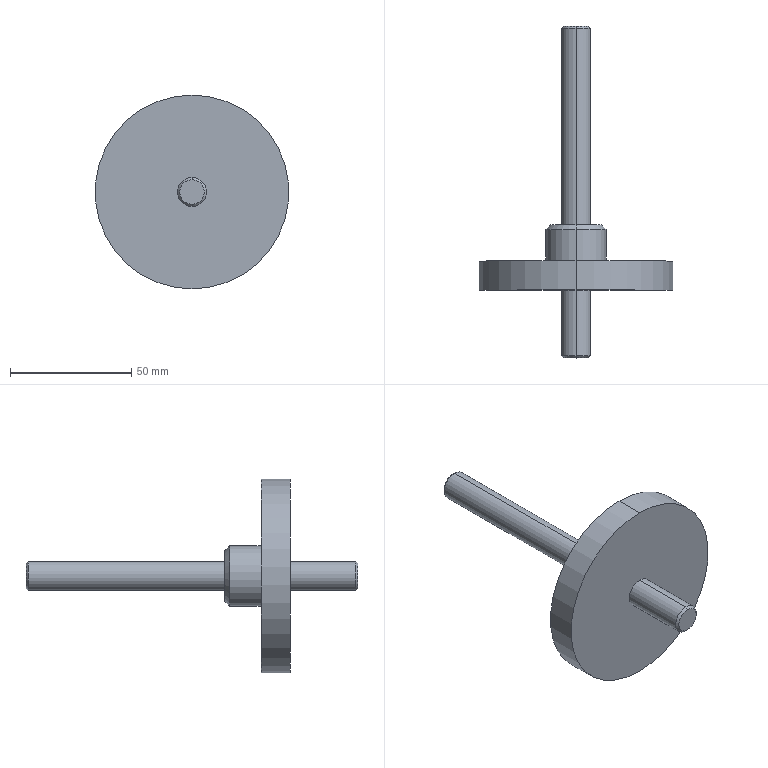Part | SolidWorks | features ICE 2, StudWizard 2, Chamfer 1, Extrusion 1 | 1 solid | 19 faces | box 80 x 137 x 80 mm | volume 79942 mm3 | cylinder 8 | cone 6 | plane 5 | commonest cylinder face diameters 12 x4 25 x2 80 x2
STEP:
#1=CARTESIAN_POINT('',(0.,27.,10.5));
#2=VERTEX_POINT('',#1);
#3=CARTESIAN_POINT('',(0.,27.,-10.5));
#4=VERTEX_POINT('',#3);
#5=CARTESIAN_POINT('',(0.,27.,0.));
#6=DIRECTION('',(0.,1.,0.));
#7=DIRECTION('',(0.,0.,1.));
#8=AXIS2_PLACEMENT_3D('',#5,#6,#7);
#9=CIRCLE('',#8,10.5);
#10=EDGE_CURVE('',#2,#4,#9,.T.);
#11=ORIENTED_EDGE('',*,*,#10,.F.);
#12=CARTESIAN_POINT('',(0.,25.,12.5));
#13=VERTEX_POINT('',#12);
#14=CARTESIAN_POINT('',(0.,27.,10.5));
#15=DIRECTION('',(0.,-0.7071,0.7071));
#16=VECTOR('',#15,1000.);
#17=LINE('',#14,#16);
#18=EDGE_CURVE('',#2,#13,#17,.T.);
#19=ORIENTED_EDGE('',*,*,#18,.T.);
#20=CARTESIAN_POINT('',(0.,25.,-12.5));
#21=VERTEX_POINT('',#20);
#22=CARTESIAN_POINT('',(0.,25.,0.));
#23=DIRECTION('',(0.,-1.,0.));
#24=DIRECTION('',(0.,0.,1.));
#25=AXIS2_PLACEMENT_3D('',#22,#23,#24);
#26=CIRCLE('',#25,12.5);
#27=EDGE_CURVE('',#21,#13,#26,.T.);
#28=ORIENTED_EDGE('',*,*,#27,.F.);
#29=CARTESIAN_POINT('',(0.,27.,-10.5));
#30=DIRECTION('',(0.,-0.7071,-0.7071));
#31=VECTOR('',#30,1000.);
#32=LINE('',#29,#31);
#33=EDGE_CURVE('',#4,#21,#32,.T.);
#34=ORIENTED_EDGE('',*,*,#33,.F.);
#35=EDGE_LOOP('',(#11,#19,#28,#34));
#36=FACE_OUTER_BOUND('',#35,.T.);
#37=CARTESIAN_POINT('',(0.,27.,0.));
#38=DIRECTION('',(0.,-1.,0.));
#39=DIRECTION('',(0.,0.,-1.));
#40=AXIS2_PLACEMENT_3D('',#37,#38,#39);
#41=CONICAL_SURFACE('',#40,10.5,0.7854);
#42=ADVANCED_FACE('',(#36),#41,.T.);
#43=CARTESIAN_POINT('',(0.,-28.,5.053));
#44=VERTEX_POINT('',#43);
#45=CARTESIAN_POINT('',(0.,-28.,-5.053));
#46=VERTEX_POINT('',#45);
#47=CARTESIAN_POINT('',(0.,-28.,0.));
#48=DIRECTION('',(0.,1.,0.));
#49=DIRECTION('',(0.,0.,1.));
#50=AXIS2_PLACEMENT_3D('',#47,#48,#49);
#51=CIRCLE('',#50,5.053);
#52=EDGE_CURVE('',#44,#46,#51,.T.);
#53=ORIENTED_EDGE('',*,*,#52,.T.);
#54=CARTESIAN_POINT('',(0.,-27.053,-6.));
#55=VERTEX_POINT('',#54);
#56=CARTESIAN_POINT('',(0.,-28.,-5.053));
#57=DIRECTION('',(0.,0.7071,-0.7071));
#58=VECTOR('',#57,1000.);
#59=LINE('',#56,#58);
#60=EDGE_CURVE('',#46,#55,#59,.T.);
#61=ORIENTED_EDGE('',*,*,#60,.T.);
#62=CARTESIAN_POINT('',(0.,-27.053,6.));
#63=VERTEX_POINT('',#62);
#64=CARTESIAN_POINT('',(0.,-27.053,0.));
#65=DIRECTION('',(0.,1.,0.));
#66=DIRECTION('',(0.,0.,1.));
#67=AXIS2_PLACEMENT_3D('',#64,#65,#66);
#68=CIRCLE('',#67,6.);
#69=EDGE_CURVE('',#63,#55,#68,.T.);
#70=ORIENTED_EDGE('',*,*,#69,.F.);
#71=CARTESIAN_POINT('',(0.,-28.,5.053));
#72=DIRECTION('',(0.,0.7071,0.7071));
#73=VECTOR('',#72,1000.);
#74=LINE('',#71,#73);
#75=EDGE_CURVE('',#44,#63,#74,.T.);
#76=ORIENTED_EDGE('',*,*,#75,.F.);
#77=EDGE_LOOP('',(#53,#61,#70,#76));
#78=FACE_OUTER_BOUND('',#77,.T.);
#79=CARTESIAN_POINT('',(0.,-28.,0.));
#80=DIRECTION('',(0.,1.,0.));
#81=DIRECTION('',(0.,0.,1.));
#82=AXIS2_PLACEMENT_3D('',#79,#80,#81);
#83=CONICAL_SURFACE('',#82,5.053,0.7854);
#84=ADVANCED_FACE('',(#78),#83,.T.);
#85=ORIENTED_EDGE('',*,*,#69,.T.);
#86=CARTESIAN_POINT('',(0.,0.,-6.));
#87=VERTEX_POINT('',#86);
#88=CARTESIAN_POINT('',(0.,-28.,-6.));
#89=DIRECTION('',(0.,1.,0.));
#90=VECTOR('',#89,1000.);
#91=LINE('',#88,#90);
#92=EDGE_CURVE('',#55,#87,#91,.T.);
#93=ORIENTED_EDGE('',*,*,#92,.T.);
#94=CARTESIAN_POINT('',(0.,0.,6.));
#95=VERTEX_POINT('',#94);
#96=CARTESIAN_POINT('',(0.,0.,0.));
#97=DIRECTION('',(0.,1.,0.));
#98=DIRECTION('',(0.,0.,1.));
#99=AXIS2_PLACEMENT_3D('',#96,#97,#98);
#100=CIRCLE('',#99,6.);
#101=EDGE_CURVE('',#95,#87,#100,.T.);
#102=ORIENTED_EDGE('',*,*,#101,.F.);
#103=CARTESIAN_POINT('',(0.,-28.,6.));
#104=DIRECTION('',(0.,1.,0.));
#105=VECTOR('',#104,1000.);
#106=LINE('',#103,#105);
#107=EDGE_CURVE('',#63,#95,#106,.T.);
#108=ORIENTED_EDGE('',*,*,#107,.F.);
#109=EDGE_LOOP('',(#85,#93,#102,#108));
#110=FACE_OUTER_BOUND('',#109,.T.);
#111=CARTESIAN_POINT('',(0.,-28.,0.));
#112=DIRECTION('',(0.,1.,0.));
#113=DIRECTION('',(0.,0.,1.));
#114=AXIS2_PLACEMENT_3D('',#111,#112,#113);
#115=CYLINDRICAL_SURFACE('',#114,6.);
#116=ADVANCED_FACE('',(#110),#115,.T.);
#117=CARTESIAN_POINT('',(0.,109.,-5.053));
#118=VERTEX_POINT('',#117);
#119=CARTESIAN_POINT('',(0.,109.,5.053));
#120=VERTEX_POINT('',#119);
#121=CARTESIAN_POINT('',(0.,109.,0.));
#122=DIRECTION('',(0.,-1.,0.));
#123=DIRECTION('',(0.,0.,-1.));
#124=AXIS2_PLACEMENT_3D('',#121,#122,#123);
#125=CIRCLE('',#124,5.053);
#126=EDGE_CURVE('',#118,#120,#125,.T.);
#127=ORIENTED_EDGE('',*,*,#126,.T.);
#128=CARTESIAN_POINT('',(0.,108.053,6.));
#129=VERTEX_POINT('',#128);
#130=CARTESIAN_POINT('',(0.,109.,5.053));
#131=DIRECTION('',(0.,-0.7071,0.7071));
#132=VECTOR('',#131,1000.);
#133=LINE('',#130,#132);
#134=EDGE_CURVE('',#120,#129,#133,.T.);
#135=ORIENTED_EDGE('',*,*,#134,.T.);
#136=CARTESIAN_POINT('',(0.,108.053,-6.));
#137=VERTEX_POINT('',#136);
#138=CARTESIAN_POINT('',(0.,108.053,0.));
#139=DIRECTION('',(0.,-1.,0.));
#140=DIRECTION('',(0.,0.,-1.));
#141=AXIS2_PLACEMENT_3D('',#138,#139,#140);
#142=CIRCLE('',#141,6.);
#143=EDGE_CURVE('',#137,#129,#142,.T.);
#144=ORIENTED_EDGE('',*,*,#143,.F.);
#145=CARTESIAN_POINT('',(0.,109.,-5.053));
#146=DIRECTION('',(0.,-0.7071,-0.7071));
#147=VECTOR('',#146,1000.);
#148=LINE('',#145,#147);
#149=EDGE_CURVE('',#118,#137,#148,.T.);
#150=ORIENTED_EDGE('',*,*,#149,.F.);
#151=EDGE_LOOP('',(#127,#135,#144,#150));
#152=FACE_OUTER_BOUND('',#151,.T.);
#153=CARTESIAN_POINT('',(0.,109.,0.));
#154=DIRECTION('',(0.,-1.,0.));
#155=DIRECTION('',(0.,0.,-1.));
#156=AXIS2_PLACEMENT_3D('',#153,#154,#155);
#157=CONICAL_SURFACE('',#156,5.053,0.7854);
#158=ADVANCED_FACE('',(#152),#157,.T.);
#159=ORIENTED_EDGE('',*,*,#143,.T.);
#160=CARTESIAN_POINT('',(0.,27.,6.));
#161=VERTEX_POINT('',#160);
#162=CARTESIAN_POINT('',(0.,109.,6.));
#163=DIRECTION('',(0.,-1.,0.));
#164=VECTOR('',#163,1000.);
#165=LINE('',#162,#164);
#166=EDGE_CURVE('',#129,#161,#165,.T.);
#167=ORIENTED_EDGE('',*,*,#166,.T.);
#168=CARTESIAN_POINT('',(0.,27.,-6.));
#169=VERTEX_POINT('',#168);
#170=CARTESIAN_POINT('',(0.,27.,0.));
#171=DIRECTION('',(0.,-1.,0.));
#172=DIRECTION('',(0.,0.,-1.));
#173=AXIS2_PLACEMENT_3D('',#170,#171,#172);
#174=CIRCLE('',#173,6.);
#175=EDGE_CURVE('',#169,#161,#174,.T.);
#176=ORIENTED_EDGE('',*,*,#175,.F.);
#177=CARTESIAN_POINT('',(0.,109.,-6.));
#178=DIRECTION('',(0.,-1.,0.));
#179=VECTOR('',#178,1000.);
#180=LINE('',#177,#179);
#181=EDGE_CURVE('',#137,#169,#180,.T.);
#182=ORIENTED_EDGE('',*,*,#181,.F.);
#183=EDGE_LOOP('',(#159,#167,#176,#182));
#184=FACE_OUTER_BOUND('',#183,.T.);
#185=CARTESIAN_POINT('',(0.,109.,0.));
#186=DIRECTION('',(0.,-1.,0.));
#187=DIRECTION('',(0.,0.,-1.));
#188=AXIS2_PLACEMENT_3D('',#185,#186,#187);
#189=CYLINDRICAL_SURFACE('',#188,6.);
#190=ADVANCED_FACE('',(#184),#189,.T.);
#191=ORIENTED_EDGE('',*,*,#27,.T.);
#192=CARTESIAN_POINT('',(0.,12.,12.5));
#193=VERTEX_POINT('',#192);
#194=CARTESIAN_POINT('',(0.,27.,12.5));
#195=DIRECTION('',(0.,-1.,0.));
#196=VECTOR('',#195,1000.);
#197=LINE('',#194,#196);
#198=EDGE_CURVE('',#13,#193,#197,.T.);
#199=ORIENTED_EDGE('',*,*,#198,.T.);
#200=CARTESIAN_POINT('',(0.,12.,-12.5));
#201=VERTEX_POINT('',#200);
#202=CARTESIAN_POINT('',(0.,12.,0.));
#203=DIRECTION('',(0.,1.,0.));
#204=DIRECTION('',(0.,0.,1.));
#205=AXIS2_PLACEMENT_3D('',#202,#203,#204);
#206=CIRCLE('',#205,12.5);
#207=EDGE_CURVE('',#193,#201,#206,.T.);
#208=ORIENTED_EDGE('',*,*,#207,.T.);
#209=CARTESIAN_POINT('',(0.,27.,-12.5));
#210=DIRECTION('',(0.,-1.,0.));
#211=VECTOR('',#210,1000.);
#212=LINE('',#209,#211);
#213=EDGE_CURVE('',#21,#201,#212,.T.);
#214=ORIENTED_EDGE('',*,*,#213,.F.);
#215=EDGE_LOOP('',(#191,#199,#208,#214));
#216=FACE_OUTER_BOUND('',#215,.T.);
#217=CARTESIAN_POINT('',(0.,27.,0.));
#218=DIRECTION('',(0.,-1.,0.));
#219=DIRECTION('',(0.,0.,-1.));
#220=AXIS2_PLACEMENT_3D('',#217,#218,#219);
#221=CYLINDRICAL_SURFACE('',#220,12.5);
#222=ADVANCED_FACE('',(#216),#221,.T.);
#223=CARTESIAN_POINT('',(0.,12.,40.));
#224=VERTEX_POINT('',#223);
#225=CARTESIAN_POINT('',(0.,12.,-40.));
#226=VERTEX_POINT('',#225);
#227=CARTESIAN_POINT('',(0.,12.,0.));
#228=DIRECTION('',(0.,1.,0.));
#229=DIRECTION('',(0.,0.,1.));
#230=AXIS2_PLACEMENT_3D('',#227,#228,#229);
#231=CIRCLE('',#230,40.);
#232=EDGE_CURVE('',#224,#226,#231,.T.);
#233=ORIENTED_EDGE('',*,*,#232,.F.);
#234=CARTESIAN_POINT('',(0.,0.,40.));
#235=VERTEX_POINT('',#234);
#236=CARTESIAN_POINT('',(0.,12.,40.));
#237=DIRECTION('',(0.,-1.,0.));
#238=VECTOR('',#237,1000.);
#239=LINE('',#236,#238);
#240=EDGE_CURVE('',#224,#235,#239,.T.);
#241=ORIENTED_EDGE('',*,*,#240,.T.);
#242=CARTESIAN_POINT('',(0.,0.,-40.));
#243=VERTEX_POINT('',#242);
#244=CARTESIAN_POINT('',(0.,0.,0.));
#245=DIRECTION('',(0.,1.,0.));
#246=DIRECTION('',(0.,0.,1.));
#247=AXIS2_PLACEMENT_3D('',#244,#245,#246);
#248=CIRCLE('',#247,40.);
#249=EDGE_CURVE('',#235,#243,#248,.T.);
#250=ORIENTED_EDGE('',*,*,#249,.T.);
#251=CARTESIAN_POINT('',(0.,12.,-40.));
#252=DIRECTION('',(0.,-1.,0.));
#253=VECTOR('',#252,1000.);
#254=LINE('',#251,#253);
#255=EDGE_CURVE('',#226,#243,#254,.T.);
#256=ORIENTED_EDGE('',*,*,#255,.F.);
#257=EDGE_LOOP('',(#233,#241,#250,#256));
#258=FACE_OUTER_BOUND('',#257,.T.);
#259=CARTESIAN_POINT('',(0.,12.,0.));
#260=DIRECTION('',(0.,-1.,0.));
#261=DIRECTION('',(0.,0.,-1.));
#262=AXIS2_PLACEMENT_3D('',#259,#260,#261);
#263=CYLINDRICAL_SURFACE('',#262,40.);
#264=ADVANCED_FACE('',(#258),#263,.T.);
#265=ORIENTED_EDGE('',*,*,#240,.F.);
#266=CARTESIAN_POINT('',(0.,12.,0.));
#267=DIRECTION('',(0.,1.,0.));
#268=DIRECTION('',(0.,0.,1.));
#269=AXIS2_PLACEMENT_3D('',#266,#267,#268);
#270=CIRCLE('',#269,40.);
#271=EDGE_CURVE('',#226,#224,#270,.T.);
#272=ORIENTED_EDGE('',*,*,#271,.F.);
#273=ORIENTED_EDGE('',*,*,#255,.T.);
#274=CARTESIAN_POINT('',(0.,0.,0.));
#275=DIRECTION('',(0.,1.,0.));
#276=DIRECTION('',(0.,0.,1.));
#277=AXIS2_PLACEMENT_3D('',#274,#275,#276);
#278=CIRCLE('',#277,40.);
#279=EDGE_CURVE('',#243,#235,#278,.T.);
#280=ORIENTED_EDGE('',*,*,#279,.T.);
#281=EDGE_LOOP('',(#265,#272,#273,#280));
#282=FACE_OUTER_BOUND('',#281,.T.);
#283=CARTESIAN_POINT('',(0.,12.,0.));
#284=DIRECTION('',(0.,-1.,0.));
#285=DIRECTION('',(0.,0.,-1.));
#286=AXIS2_PLACEMENT_3D('',#283,#284,#285);
#287=CYLINDRICAL_SURFACE('',#286,40.);
#288=ADVANCED_FACE('',(#282),#287,.T.);
#289=CARTESIAN_POINT('',(0.,12.,0.));
#290=DIRECTION('',(0.,1.,0.));
#291=DIRECTION('',(0.,0.,1.));
#292=AXIS2_PLACEMENT_3D('',#289,#290,#291);
#293=CIRCLE('',#292,12.5);
#294=EDGE_CURVE('',#201,#193,#293,.T.);
#295=ORIENTED_EDGE('',*,*,#294,.F.);
#296=ORIENTED_EDGE('',*,*,#207,.F.);
#297=EDGE_LOOP('',(#295,#296));
#298=FACE_BOUND('',#297,.T.);
#299=ORIENTED_EDGE('',*,*,#271,.T.);
#300=ORIENTED_EDGE('',*,*,#232,.T.);
#301=EDGE_LOOP('',(#299,#300));
#302=FACE_OUTER_BOUND('',#301,.T.);
#303=CARTESIAN_POINT('',(0.,12.,0.));
#304=DIRECTION('',(0.,1.,0.));
#305=DIRECTION('',(0.,0.,1.));
#306=AXIS2_PLACEMENT_3D('',#303,#304,#305);
#307=PLANE('',#306);
#308=ADVANCED_FACE('',(#298,#302),#307,.T.);
#309=ORIENTED_EDGE('',*,*,#279,.F.);
#310=ORIENTED_EDGE('',*,*,#249,.F.);
#311=EDGE_LOOP('',(#309,#310));
#312=FACE_OUTER_BOUND('',#311,.T.);
#313=ORIENTED_EDGE('',*,*,#101,.T.);
#314=CARTESIAN_POINT('',(0.,0.,0.));
#315=DIRECTION('',(0.,1.,0.));
#316=DIRECTION('',(0.,0.,1.));
#317=AXIS2_PLACEMENT_3D('',#314,#315,#316);
#318=CIRCLE('',#317,6.);
#319=EDGE_CURVE('',#87,#95,#318,.T.);
#320=ORIENTED_EDGE('',*,*,#319,.T.);
#321=EDGE_LOOP('',(#313,#320));
#322=FACE_BOUND('',#321,.T.);
#323=CARTESIAN_POINT('',(0.,0.,0.));
#324=DIRECTION('',(0.,1.,0.));
#325=DIRECTION('',(0.,0.,1.));
#326=AXIS2_PLACEMENT_3D('',#323,#324,#325);
#327=PLANE('',#326);
#328=ADVANCED_FACE('',(#312,#322),#327,.F.);
#329=ORIENTED_EDGE('',*,*,#198,.F.);
#330=CARTESIAN_POINT('',(0.,25.,0.));
#331=DIRECTION('',(0.,-1.,0.));
#332=DIRECTION('',(0.,0.,1.));
#333=AXIS2_PLACEMENT_3D('',#330,#331,#332);
#334=CIRCLE('',#333,12.5);
#335=EDGE_CURVE('',#13,#21,#334,.T.);
#336=ORIENTED_EDGE('',*,*,#335,.T.);
#337=ORIENTED_EDGE('',*,*,#213,.T.);
#338=ORIENTED_EDGE('',*,*,#294,.T.);
#339=EDGE_LOOP('',(#329,#336,#337,#338));
#340=FACE_OUTER_BOUND('',#339,.T.);
#341=CARTESIAN_POINT('',(0.,27.,0.));
#342=DIRECTION('',(0.,-1.,0.));
#343=DIRECTION('',(0.,0.,-1.));
#344=AXIS2_PLACEMENT_3D('',#341,#342,#343);
#345=CYLINDRICAL_SURFACE('',#344,12.5);
#346=ADVANCED_FACE('',(#340),#345,.T.);
#347=CARTESIAN_POINT('',(0.,27.,0.));
#348=DIRECTION('',(0.,1.,0.));
#349=DIRECTION('',(0.,0.,1.));
#350=AXIS2_PLACEMENT_3D('',#347,#348,#349);
#351=CIRCLE('',#350,10.5);
#352=EDGE_CURVE('',#4,#2,#351,.T.);
#353=ORIENTED_EDGE('',*,*,#352,.T.);
#354=ORIENTED_EDGE('',*,*,#10,.T.);
#355=EDGE_LOOP('',(#353,#354));
#356=FACE_OUTER_BOUND('',#355,.T.);
#357=ORIENTED_EDGE('',*,*,#175,.T.);
#358=CARTESIAN_POINT('',(0.,27.,0.));
#359=DIRECTION('',(0.,-1.,0.));
#360=DIRECTION('',(0.,0.,-1.));
#361=AXIS2_PLACEMENT_3D('',#358,#359,#360);
#362=CIRCLE('',#361,6.);
#363=EDGE_CURVE('',#161,#169,#362,.T.);
#364=ORIENTED_EDGE('',*,*,#363,.T.);
#365=EDGE_LOOP('',(#357,#364));
#366=FACE_BOUND('',#365,.T.);
#367=CARTESIAN_POINT('',(0.,27.,0.));
#368=DIRECTION('',(0.,1.,0.));
#369=DIRECTION('',(0.,0.,1.));
#370=AXIS2_PLACEMENT_3D('',#367,#368,#369);
#371=PLANE('',#370);
#372=ADVANCED_FACE('',(#356,#366),#371,.T.);
#373=ORIENTED_EDGE('',*,*,#166,.F.);
#374=CARTESIAN_POINT('',(0.,108.053,0.));
#375=DIRECTION('',(0.,-1.,0.));
#376=DIRECTION('',(0.,0.,-1.));
#377=AXIS2_PLACEMENT_3D('',#374,#375,#376);
#378=CIRCLE('',#377,6.);
#379=EDGE_CURVE('',#129,#137,#378,.T.);
#380=ORIENTED_EDGE('',*,*,#379,.T.);
#381=ORIENTED_EDGE('',*,*,#181,.T.);
#382=ORIENTED_EDGE('',*,*,#363,.F.);
#383=EDGE_LOOP('',(#373,#380,#381,#382));
#384=FACE_OUTER_BOUND('',#383,.T.);
#385=CARTESIAN_POINT('',(0.,109.,0.));
#386=DIRECTION('',(0.,-1.,0.));
#387=DIRECTION('',(0.,0.,-1.));
#388=AXIS2_PLACEMENT_3D('',#385,#386,#387);
#389=CYLINDRICAL_SURFACE('',#388,6.);
#390=ADVANCED_FACE('',(#384),#389,.T.);
#391=ORIENTED_EDGE('',*,*,#134,.F.);
#392=CARTESIAN_POINT('',(0.,109.,0.));
#393=DIRECTION('',(0.,-1.,0.));
#394=DIRECTION('',(0.,0.,-1.));
#395=AXIS2_PLACEMENT_3D('',#392,#393,#394);
#396=CIRCLE('',#395,5.053);
#397=EDGE_CURVE('',#120,#118,#396,.T.);
#398=ORIENTED_EDGE('',*,*,#397,.T.);
#399=ORIENTED_EDGE('',*,*,#149,.T.);
#400=ORIENTED_EDGE('',*,*,#379,.F.);
#401=EDGE_LOOP('',(#391,#398,#399,#400));
#402=FACE_OUTER_BOUND('',#401,.T.);
#403=CARTESIAN_POINT('',(0.,109.,0.));
#404=DIRECTION('',(0.,-1.,0.));
#405=DIRECTION('',(0.,0.,-1.));
#406=AXIS2_PLACEMENT_3D('',#403,#404,#405);
#407=CONICAL_SURFACE('',#406,5.053,0.7854);
#408=ADVANCED_FACE('',(#402),#407,.T.);
#409=ORIENTED_EDGE('',*,*,#126,.F.);
#410=ORIENTED_EDGE('',*,*,#397,.F.);
#411=EDGE_LOOP('',(#409,#410));
#412=FACE_OUTER_BOUND('',#411,.T.);
#413=CARTESIAN_POINT('',(0.,109.,0.));
#414=DIRECTION('',(0.,1.,0.));
#415=DIRECTION('',(0.,0.,1.));
#416=AXIS2_PLACEMENT_3D('',#413,#414,#415);
#417=PLANE('',#416);
#418=ADVANCED_FACE('',(#412),#417,.T.);
#419=ORIENTED_EDGE('',*,*,#92,.F.);
#420=CARTESIAN_POINT('',(0.,-27.053,0.));
#421=DIRECTION('',(0.,1.,0.));
#422=DIRECTION('',(0.,0.,1.));
#423=AXIS2_PLACEMENT_3D('',#420,#421,#422);
#424=CIRCLE('',#423,6.);
#425=EDGE_CURVE('',#55,#63,#424,.T.);
#426=ORIENTED_EDGE('',*,*,#425,.T.);
#427=ORIENTED_EDGE('',*,*,#107,.T.);
#428=ORIENTED_EDGE('',*,*,#319,.F.);
#429=EDGE_LOOP('',(#419,#426,#427,#428));
#430=FACE_OUTER_BOUND('',#429,.T.);
#431=CARTESIAN_POINT('',(0.,-28.,0.));
#432=DIRECTION('',(0.,1.,0.));
#433=DIRECTION('',(0.,0.,1.));
#434=AXIS2_PLACEMENT_3D('',#431,#432,#433);
#435=CYLINDRICAL_SURFACE('',#434,6.);
#436=ADVANCED_FACE('',(#430),#435,.T.);
#437=ORIENTED_EDGE('',*,*,#60,.F.);
#438=CARTESIAN_POINT('',(0.,-28.,0.));
#439=DIRECTION('',(0.,1.,0.));
#440=DIRECTION('',(0.,0.,1.));
#441=AXIS2_PLACEMENT_3D('',#438,#439,#440);
#442=CIRCLE('',#441,5.053);
#443=EDGE_CURVE('',#46,#44,#442,.T.);
#444=ORIENTED_EDGE('',*,*,#443,.T.);
#445=ORIENTED_EDGE('',*,*,#75,.T.);
#446=ORIENTED_EDGE('',*,*,#425,.F.);
#447=EDGE_LOOP('',(#437,#444,#445,#446));
#448=FACE_OUTER_BOUND('',#447,.T.);
#449=CARTESIAN_POINT('',(0.,-28.,0.));
#450=DIRECTION('',(0.,1.,0.));
#451=DIRECTION('',(0.,0.,1.));
#452=AXIS2_PLACEMENT_3D('',#449,#450,#451);
#453=CONICAL_SURFACE('',#452,5.053,0.7854);
#454=ADVANCED_FACE('',(#448),#453,.T.);
#455=ORIENTED_EDGE('',*,*,#52,.F.);
#456=ORIENTED_EDGE('',*,*,#443,.F.);
#457=EDGE_LOOP('',(#455,#456));
#458=FACE_OUTER_BOUND('',#457,.T.);
#459=CARTESIAN_POINT('',(0.,-28.,0.));
#460=DIRECTION('',(0.,1.,0.));
#461=DIRECTION('',(0.,0.,1.));
#462=AXIS2_PLACEMENT_3D('',#459,#460,#461);
#463=PLANE('',#462);
#464=ADVANCED_FACE('',(#458),#463,.F.);
#465=ORIENTED_EDGE('',*,*,#18,.F.);
#466=ORIENTED_EDGE('',*,*,#352,.F.);
#467=ORIENTED_EDGE('',*,*,#33,.T.);
#468=ORIENTED_EDGE('',*,*,#335,.F.);
#469=EDGE_LOOP('',(#465,#466,#467,#468));
#470=FACE_OUTER_BOUND('',#469,.T.);
#471=CARTESIAN_POINT('',(0.,27.,0.));
#472=DIRECTION('',(0.,-1.,0.));
#473=DIRECTION('',(0.,0.,-1.));
#474=AXIS2_PLACEMENT_3D('',#471,#472,#473);
#475=CONICAL_SURFACE('',#474,10.5,0.7854);
#476=ADVANCED_FACE('',(#470),#475,.T.);
#477=CLOSED_SHELL('',(#42,#84,#116,#158,#190,#222,#264,#288,#308,#328,#346,#372,#390,#408,#418,#436,#454,#464,#476));
#478=MANIFOLD_SOLID_BREP('',#477);
#479=CARTESIAN_POINT('',(0.,0.,0.));
#480=DIRECTION('',(0.,0.,1.));
#481=DIRECTION('',(1.,0.,0.));
#482=AXIS2_PLACEMENT_3D('',#479,#480,#481);
#483=(LENGTH_UNIT()NAMED_UNIT(*)SI_UNIT(.MILLI.,.METRE.));
#484=UNCERTAINTY_MEASURE_WITH_UNIT(LENGTH_MEASURE(0.00001),#483,'','');
#485=(NAMED_UNIT(*)PLANE_ANGLE_UNIT()SI_UNIT($,.RADIAN.));
#486=(NAMED_UNIT(*)SI_UNIT($,.STERADIAN.)SOLID_ANGLE_UNIT());
#487=(GEOMETRIC_REPRESENTATION_CONTEXT(3)GLOBAL_UNCERTAINTY_ASSIGNED_CONTEXT((#484))GLOBAL_UNIT_ASSIGNED_CONTEXT((#483,#485,#486))REPRESENTATION_CONTEXT('',''));
#488=ADVANCED_BREP_SHAPE_REPRESENTATION('',(#478,#482),#487);